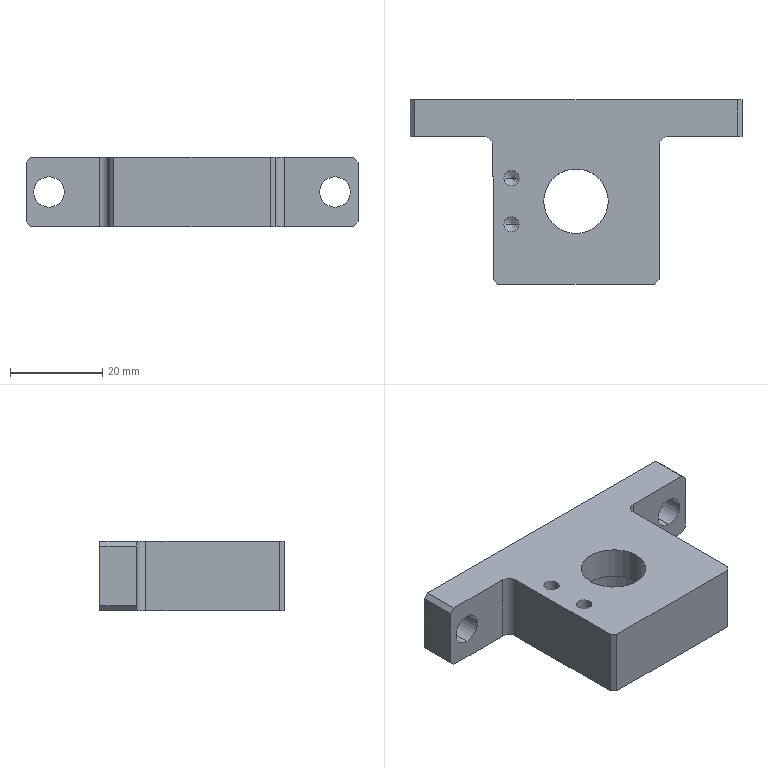Part | STEP file | FBDS-CS-018 | 1 solid | 47 faces | box 72 x 40 x 15 mm | volume 21999 mm3 | cylinder 18 | plane 17 | cone 12 | commonest cylinder face diameters 2.5 x4 3.3 x4 6.6 x4 4 x2 14 x2 18 x2
STEP:
#1=CARTESIAN_POINT('',(12.25,-2.,0.275));
#2=VERTEX_POINT('',#1);
#3=CARTESIAN_POINT('',(9.75,-2.,0.275));
#4=VERTEX_POINT('',#3);
#5=CARTESIAN_POINT('',(11.,-2.,0.275));
#6=DIRECTION('',(0.,0.,-1.));
#7=DIRECTION('',(-1.,0.,0.));
#8=AXIS2_PLACEMENT_3D('',#5,#6,#7);
#9=CIRCLE('',#8,1.25);
#10=EDGE_CURVE('',#2,#4,#9,.T.);
#11=ORIENTED_EDGE('',*,*,#10,.F.);
#12=CARTESIAN_POINT('',(12.525,-2.,0.));
#13=VERTEX_POINT('',#12);
#14=CARTESIAN_POINT('',(12.525,-2.,0.));
#15=DIRECTION('',(0.7071,0.,-0.7071));
#16=VECTOR('',#15,1000.);
#17=LINE('',#14,#16);
#18=EDGE_CURVE('',#2,#13,#17,.T.);
#19=ORIENTED_EDGE('',*,*,#18,.T.);
#20=CARTESIAN_POINT('',(9.475,-2.,0.));
#21=VERTEX_POINT('',#20);
#22=CARTESIAN_POINT('',(11.,-2.,0.));
#23=DIRECTION('',(0.,0.,-1.));
#24=DIRECTION('',(-1.,0.,0.));
#25=AXIS2_PLACEMENT_3D('',#22,#23,#24);
#26=CIRCLE('',#25,1.525);
#27=EDGE_CURVE('',#13,#21,#26,.T.);
#28=ORIENTED_EDGE('',*,*,#27,.T.);
#29=CARTESIAN_POINT('',(9.475,-2.,0.));
#30=DIRECTION('',(-0.7071,0.,-0.7071));
#31=VECTOR('',#30,1000.);
#32=LINE('',#29,#31);
#33=EDGE_CURVE('',#4,#21,#32,.T.);
#34=ORIENTED_EDGE('',*,*,#33,.F.);
#35=EDGE_LOOP('',(#11,#19,#28,#34));
#36=FACE_OUTER_BOUND('',#35,.T.);
#37=CARTESIAN_POINT('',(11.,-2.,0.));
#38=DIRECTION('',(0.,0.,-1.));
#39=DIRECTION('',(-1.,0.,0.));
#40=AXIS2_PLACEMENT_3D('',#37,#38,#39);
#41=CONICAL_SURFACE('',#40,1.525,0.7854);
#42=ADVANCED_FACE('',(#36),#41,.F.);
#43=CARTESIAN_POINT('',(12.25,-2.,7.5));
#44=VERTEX_POINT('',#43);
#45=CARTESIAN_POINT('',(9.75,-2.,7.5));
#46=VERTEX_POINT('',#45);
#47=CARTESIAN_POINT('',(11.,-2.,7.5));
#48=DIRECTION('',(0.,0.,-1.));
#49=DIRECTION('',(-1.,0.,0.));
#50=AXIS2_PLACEMENT_3D('',#47,#48,#49);
#51=CIRCLE('',#50,1.25);
#52=EDGE_CURVE('',#44,#46,#51,.T.);
#53=ORIENTED_EDGE('',*,*,#52,.F.);
#54=CARTESIAN_POINT('',(12.25,-2.,0.));
#55=DIRECTION('',(0.,0.,-1.));
#56=VECTOR('',#55,1000.);
#57=LINE('',#54,#56);
#58=EDGE_CURVE('',#44,#2,#57,.T.);
#59=ORIENTED_EDGE('',*,*,#58,.T.);
#60=ORIENTED_EDGE('',*,*,#10,.T.);
#61=CARTESIAN_POINT('',(9.75,-2.,0.));
#62=DIRECTION('',(0.,0.,-1.));
#63=VECTOR('',#62,1000.);
#64=LINE('',#61,#63);
#65=EDGE_CURVE('',#46,#4,#64,.T.);
#66=ORIENTED_EDGE('',*,*,#65,.F.);
#67=EDGE_LOOP('',(#53,#59,#60,#66));
#68=FACE_OUTER_BOUND('',#67,.T.);
#69=CARTESIAN_POINT('',(11.,-2.,0.));
#70=DIRECTION('',(0.,0.,-1.));
#71=DIRECTION('',(-1.,0.,0.));
#72=AXIS2_PLACEMENT_3D('',#69,#70,#71);
#73=CYLINDRICAL_SURFACE('',#72,1.25);
#74=ADVANCED_FACE('',(#68),#73,.F.);
#75=CARTESIAN_POINT('',(11.,-2.,8.251));
#76=VERTEX_POINT('',#75);
#77=CARTESIAN_POINT('',(9.75,-2.,7.5));
#78=DIRECTION('',(-0.8572,0.,-0.515));
#79=VECTOR('',#78,1000.);
#80=LINE('',#77,#79);
#81=EDGE_CURVE('',#76,#46,#80,.T.);
#82=ORIENTED_EDGE('',*,*,#81,.F.);
#83=CARTESIAN_POINT('',(12.25,-2.,7.5));
#84=DIRECTION('',(0.8572,0.,-0.515));
#85=VECTOR('',#84,1000.);
#86=LINE('',#83,#85);
#87=EDGE_CURVE('',#76,#44,#86,.T.);
#88=ORIENTED_EDGE('',*,*,#87,.T.);
#89=ORIENTED_EDGE('',*,*,#52,.T.);
#90=EDGE_LOOP('',(#82,#88,#89));
#91=FACE_OUTER_BOUND('',#90,.T.);
#92=CARTESIAN_POINT('',(11.,-2.,7.5));
#93=DIRECTION('',(0.,0.,-1.));
#94=DIRECTION('',(-1.,0.,0.));
#95=AXIS2_PLACEMENT_3D('',#92,#93,#94);
#96=CONICAL_SURFACE('',#95,1.25,1.03);
#97=ADVANCED_FACE('',(#91),#96,.F.);
#98=CARTESIAN_POINT('',(-9.75,-2.,0.275));
#99=VERTEX_POINT('',#98);
#100=CARTESIAN_POINT('',(-12.25,-2.,0.275));
#101=VERTEX_POINT('',#100);
#102=CARTESIAN_POINT('',(-11.,-2.,0.275));
#103=DIRECTION('',(0.,0.,-1.));
#104=DIRECTION('',(-1.,0.,0.));
#105=AXIS2_PLACEMENT_3D('',#102,#103,#104);
#106=CIRCLE('',#105,1.25);
#107=EDGE_CURVE('',#99,#101,#106,.T.);
#108=ORIENTED_EDGE('',*,*,#107,.F.);
#109=CARTESIAN_POINT('',(-9.475,-2.,0.));
#110=VERTEX_POINT('',#109);
#111=CARTESIAN_POINT('',(-9.475,-2.,0.));
#112=DIRECTION('',(0.7071,0.,-0.7071));
#113=VECTOR('',#112,1000.);
#114=LINE('',#111,#113);
#115=EDGE_CURVE('',#99,#110,#114,.T.);
#116=ORIENTED_EDGE('',*,*,#115,.T.);
#117=CARTESIAN_POINT('',(-12.525,-2.,0.));
#118=VERTEX_POINT('',#117);
#119=CARTESIAN_POINT('',(-11.,-2.,0.));
#120=DIRECTION('',(0.,0.,-1.));
#121=DIRECTION('',(-1.,0.,0.));
#122=AXIS2_PLACEMENT_3D('',#119,#120,#121);
#123=CIRCLE('',#122,1.525);
#124=EDGE_CURVE('',#110,#118,#123,.T.);
#125=ORIENTED_EDGE('',*,*,#124,.T.);
#126=CARTESIAN_POINT('',(-12.525,-2.,0.));
#127=DIRECTION('',(-0.7071,0.,-0.7071));
#128=VECTOR('',#127,1000.);
#129=LINE('',#126,#128);
#130=EDGE_CURVE('',#101,#118,#129,.T.);
#131=ORIENTED_EDGE('',*,*,#130,.F.);
#132=EDGE_LOOP('',(#108,#116,#125,#131));
#133=FACE_OUTER_BOUND('',#132,.T.);
#134=CARTESIAN_POINT('',(-11.,-2.,0.));
#135=DIRECTION('',(0.,0.,-1.));
#136=DIRECTION('',(-1.,0.,0.));
#137=AXIS2_PLACEMENT_3D('',#134,#135,#136);
#138=CONICAL_SURFACE('',#137,1.525,0.7854);
#139=ADVANCED_FACE('',(#133),#138,.F.);
#140=CARTESIAN_POINT('',(-9.75,-2.,7.5));
#141=VERTEX_POINT('',#140);
#142=CARTESIAN_POINT('',(-12.25,-2.,7.5));
#143=VERTEX_POINT('',#142);
#144=CARTESIAN_POINT('',(-11.,-2.,7.5));
#145=DIRECTION('',(0.,0.,-1.));
#146=DIRECTION('',(-1.,0.,0.));
#147=AXIS2_PLACEMENT_3D('',#144,#145,#146);
#148=CIRCLE('',#147,1.25);
#149=EDGE_CURVE('',#141,#143,#148,.T.);
#150=ORIENTED_EDGE('',*,*,#149,.F.);
#151=CARTESIAN_POINT('',(-9.75,-2.,0.));
#152=DIRECTION('',(0.,0.,-1.));
#153=VECTOR('',#152,1000.);
#154=LINE('',#151,#153);
#155=EDGE_CURVE('',#141,#99,#154,.T.);
#156=ORIENTED_EDGE('',*,*,#155,.T.);
#157=ORIENTED_EDGE('',*,*,#107,.T.);
#158=CARTESIAN_POINT('',(-12.25,-2.,0.));
#159=DIRECTION('',(0.,0.,-1.));
#160=VECTOR('',#159,1000.);
#161=LINE('',#158,#160);
#162=EDGE_CURVE('',#143,#101,#161,.T.);
#163=ORIENTED_EDGE('',*,*,#162,.F.);
#164=EDGE_LOOP('',(#150,#156,#157,#163));
#165=FACE_OUTER_BOUND('',#164,.T.);
#166=CARTESIAN_POINT('',(-11.,-2.,0.));
#167=DIRECTION('',(0.,0.,-1.));
#168=DIRECTION('',(-1.,0.,0.));
#169=AXIS2_PLACEMENT_3D('',#166,#167,#168);
#170=CYLINDRICAL_SURFACE('',#169,1.25);
#171=ADVANCED_FACE('',(#165),#170,.F.);
#172=CARTESIAN_POINT('',(-11.,-2.,8.251));
#173=VERTEX_POINT('',#172);
#174=CARTESIAN_POINT('',(-12.25,-2.,7.5));
#175=DIRECTION('',(-0.8572,0.,-0.515));
#176=VECTOR('',#175,1000.);
#177=LINE('',#174,#176);
#178=EDGE_CURVE('',#173,#143,#177,.T.);
#179=ORIENTED_EDGE('',*,*,#178,.F.);
#180=CARTESIAN_POINT('',(-9.75,-2.,7.5));
#181=DIRECTION('',(0.8572,0.,-0.515));
#182=VECTOR('',#181,1000.);
#183=LINE('',#180,#182);
#184=EDGE_CURVE('',#173,#141,#183,.T.);
#185=ORIENTED_EDGE('',*,*,#184,.T.);
#186=ORIENTED_EDGE('',*,*,#149,.T.);
#187=EDGE_LOOP('',(#179,#185,#186));
#188=FACE_OUTER_BOUND('',#187,.T.);
#189=CARTESIAN_POINT('',(-11.,-2.,7.5));
#190=DIRECTION('',(0.,0.,-1.));
#191=DIRECTION('',(-1.,0.,0.));
#192=AXIS2_PLACEMENT_3D('',#189,#190,#191);
#193=CONICAL_SURFACE('',#192,1.25,1.03);
#194=ADVANCED_FACE('',(#188),#193,.F.);
#195=CARTESIAN_POINT('',(-15.65,3.,4.9));
#196=VERTEX_POINT('',#195);
#197=CARTESIAN_POINT('',(-12.35,3.,4.9));
#198=VERTEX_POINT('',#197);
#199=CARTESIAN_POINT('',(-14.,3.,4.9));
#200=DIRECTION('',(0.,0.,1.));
#201=DIRECTION('',(1.,0.,0.));
#202=AXIS2_PLACEMENT_3D('',#199,#200,#201);
#203=CIRCLE('',#202,1.65);
#204=EDGE_CURVE('',#196,#198,#203,.T.);
#205=ORIENTED_EDGE('',*,*,#204,.F.);
#206=CARTESIAN_POINT('',(-15.65,3.,15.));
#207=VERTEX_POINT('',#206);
#208=CARTESIAN_POINT('',(-15.65,3.,15.));
#209=DIRECTION('',(0.,0.,1.));
#210=VECTOR('',#209,1000.);
#211=LINE('',#208,#210);
#212=EDGE_CURVE('',#196,#207,#211,.T.);
#213=ORIENTED_EDGE('',*,*,#212,.T.);
#214=CARTESIAN_POINT('',(-12.35,3.,15.));
#215=VERTEX_POINT('',#214);
#216=CARTESIAN_POINT('',(-14.,3.,15.));
#217=DIRECTION('',(0.,0.,1.));
#218=DIRECTION('',(1.,0.,0.));
#219=AXIS2_PLACEMENT_3D('',#216,#217,#218);
#220=CIRCLE('',#219,1.65);
#221=EDGE_CURVE('',#207,#215,#220,.T.);
#222=ORIENTED_EDGE('',*,*,#221,.T.);
#223=CARTESIAN_POINT('',(-12.35,3.,15.));
#224=DIRECTION('',(0.,0.,1.));
#225=VECTOR('',#224,1000.);
#226=LINE('',#223,#225);
#227=EDGE_CURVE('',#198,#215,#226,.T.);
#228=ORIENTED_EDGE('',*,*,#227,.F.);
#229=EDGE_LOOP('',(#205,#213,#222,#228));
#230=FACE_OUTER_BOUND('',#229,.T.);
#231=CARTESIAN_POINT('',(-14.,3.,15.));
#232=DIRECTION('',(0.,0.,1.));
#233=DIRECTION('',(1.,0.,0.));
#234=AXIS2_PLACEMENT_3D('',#231,#232,#233);
#235=CYLINDRICAL_SURFACE('',#234,1.65);
#236=ADVANCED_FACE('',(#230),#235,.F.);
#237=CARTESIAN_POINT('',(-14.,3.,3.909));
#238=VERTEX_POINT('',#237);
#239=CARTESIAN_POINT('',(-12.35,3.,4.9));
#240=DIRECTION('',(0.8572,0.,0.515));
#241=VECTOR('',#240,1000.);
#242=LINE('',#239,#241);
#243=EDGE_CURVE('',#238,#198,#242,.T.);
#244=ORIENTED_EDGE('',*,*,#243,.F.);
#245=CARTESIAN_POINT('',(-15.65,3.,4.9));
#246=DIRECTION('',(-0.8572,0.,0.515));
#247=VECTOR('',#246,1000.);
#248=LINE('',#245,#247);
#249=EDGE_CURVE('',#238,#196,#248,.T.);
#250=ORIENTED_EDGE('',*,*,#249,.T.);
#251=ORIENTED_EDGE('',*,*,#204,.T.);
#252=EDGE_LOOP('',(#244,#250,#251));
#253=FACE_OUTER_BOUND('',#252,.T.);
#254=CARTESIAN_POINT('',(-14.,3.,4.9));
#255=DIRECTION('',(0.,0.,1.));
#256=DIRECTION('',(1.,0.,0.));
#257=AXIS2_PLACEMENT_3D('',#254,#255,#256);
#258=CONICAL_SURFACE('',#257,1.65,1.03);
#259=ADVANCED_FACE('',(#253),#258,.F.);
#260=CARTESIAN_POINT('',(-15.65,-7.,4.9));
#261=VERTEX_POINT('',#260);
#262=CARTESIAN_POINT('',(-12.35,-7.,4.9));
#263=VERTEX_POINT('',#262);
#264=CARTESIAN_POINT('',(-14.,-7.,4.9));
#265=DIRECTION('',(0.,0.,1.));
#266=DIRECTION('',(1.,0.,0.));
#267=AXIS2_PLACEMENT_3D('',#264,#265,#266);
#268=CIRCLE('',#267,1.65);
#269=EDGE_CURVE('',#261,#263,#268,.T.);
#270=ORIENTED_EDGE('',*,*,#269,.F.);
#271=CARTESIAN_POINT('',(-15.65,-7.,15.));
#272=VERTEX_POINT('',#271);
#273=CARTESIAN_POINT('',(-15.65,-7.,15.));
#274=DIRECTION('',(0.,0.,1.));
#275=VECTOR('',#274,1000.);
#276=LINE('',#273,#275);
#277=EDGE_CURVE('',#261,#272,#276,.T.);
#278=ORIENTED_EDGE('',*,*,#277,.T.);
#279=CARTESIAN_POINT('',(-12.35,-7.,15.));
#280=VERTEX_POINT('',#279);
#281=CARTESIAN_POINT('',(-14.,-7.,15.));
#282=DIRECTION('',(0.,0.,1.));
#283=DIRECTION('',(1.,0.,0.));
#284=AXIS2_PLACEMENT_3D('',#281,#282,#283);
#285=CIRCLE('',#284,1.65);
#286=EDGE_CURVE('',#272,#280,#285,.T.);
#287=ORIENTED_EDGE('',*,*,#286,.T.);
#288=CARTESIAN_POINT('',(-12.35,-7.,15.));
#289=DIRECTION('',(0.,0.,1.));
#290=VECTOR('',#289,1000.);
#291=LINE('',#288,#290);
#292=EDGE_CURVE('',#263,#280,#291,.T.);
#293=ORIENTED_EDGE('',*,*,#292,.F.);
#294=EDGE_LOOP('',(#270,#278,#287,#293));
#295=FACE_OUTER_BOUND('',#294,.T.);
#296=CARTESIAN_POINT('',(-14.,-7.,15.));
#297=DIRECTION('',(0.,0.,1.));
#298=DIRECTION('',(1.,0.,0.));
#299=AXIS2_PLACEMENT_3D('',#296,#297,#298);
#300=CYLINDRICAL_SURFACE('',#299,1.65);
#301=ADVANCED_FACE('',(#295),#300,.F.);
#302=CARTESIAN_POINT('',(-14.,-7.,3.909));
#303=VERTEX_POINT('',#302);
#304=CARTESIAN_POINT('',(-12.35,-7.,4.9));
#305=DIRECTION('',(0.8572,0.,0.515));
#306=VECTOR('',#305,1000.);
#307=LINE('',#304,#306);
#308=EDGE_CURVE('',#303,#263,#307,.T.);
#309=ORIENTED_EDGE('',*,*,#308,.F.);
#310=CARTESIAN_POINT('',(-15.65,-7.,4.9));
#311=DIRECTION('',(-0.8572,0.,0.515));
#312=VECTOR('',#311,1000.);
#313=LINE('',#310,#312);
#314=EDGE_CURVE('',#303,#261,#313,.T.);
#315=ORIENTED_EDGE('',*,*,#314,.T.);
#316=ORIENTED_EDGE('',*,*,#269,.T.);
#317=EDGE_LOOP('',(#309,#315,#316));
#318=FACE_OUTER_BOUND('',#317,.T.);
#319=CARTESIAN_POINT('',(-14.,-7.,4.9));
#320=DIRECTION('',(0.,0.,1.));
#321=DIRECTION('',(1.,0.,0.));
#322=AXIS2_PLACEMENT_3D('',#319,#320,#321);
#323=CONICAL_SURFACE('',#322,1.65,1.03);
#324=ADVANCED_FACE('',(#318),#323,.F.);
#325=CARTESIAN_POINT('',(-31.,20.,10.8));
#326=VERTEX_POINT('',#325);
#327=CARTESIAN_POINT('',(-31.,20.,4.2));
#328=VERTEX_POINT('',#327);
#329=CARTESIAN_POINT('',(-31.,20.,7.5));
#330=DIRECTION('',(0.,-1.,0.));
#331=DIRECTION('',(0.,0.,-1.));
#332=AXIS2_PLACEMENT_3D('',#329,#330,#331);
#333=CIRCLE('',#332,3.3);
#334=EDGE_CURVE('',#326,#328,#333,.T.);
#335=ORIENTED_EDGE('',*,*,#334,.F.);
#336=CARTESIAN_POINT('',(-31.,12.,10.8));
#337=VERTEX_POINT('',#336);
#338=CARTESIAN_POINT('',(-31.,12.,10.8));
#339=DIRECTION('',(0.,-1.,0.));
#340=VECTOR('',#339,1000.);
#341=LINE('',#338,#340);
#342=EDGE_CURVE('',#326,#337,#341,.T.);
#343=ORIENTED_EDGE('',*,*,#342,.T.);
#344=CARTESIAN_POINT('',(-31.,12.,4.2));
#345=VERTEX_POINT('',#344);
#346=CARTESIAN_POINT('',(-31.,12.,7.5));
#347=DIRECTION('',(0.,-1.,0.));
#348=DIRECTION('',(0.,0.,-1.));
#349=AXIS2_PLACEMENT_3D('',#346,#347,#348);
#350=CIRCLE('',#349,3.3);
#351=EDGE_CURVE('',#337,#345,#350,.T.);
#352=ORIENTED_EDGE('',*,*,#351,.T.);
#353=CARTESIAN_POINT('',(-31.,12.,4.2));
#354=DIRECTION('',(0.,-1.,0.));
#355=VECTOR('',#354,1000.);
#356=LINE('',#353,#355);
#357=EDGE_CURVE('',#328,#345,#356,.T.);
#358=ORIENTED_EDGE('',*,*,#357,.F.);
#359=EDGE_LOOP('',(#335,#343,#352,#358));
#360=FACE_OUTER_BOUND('',#359,.T.);
#361=CARTESIAN_POINT('',(-31.,12.,7.5));
#362=DIRECTION('',(0.,-1.,0.));
#363=DIRECTION('',(0.,0.,-1.));
#364=AXIS2_PLACEMENT_3D('',#361,#362,#363);
#365=CYLINDRICAL_SURFACE('',#364,3.3);
#366=ADVANCED_FACE('',(#360),#365,.F.);
#367=CARTESIAN_POINT('',(31.,20.,10.8));
#368=VERTEX_POINT('',#367);
#369=CARTESIAN_POINT('',(31.,20.,4.2));
#370=VERTEX_POINT('',#369);
#371=CARTESIAN_POINT('',(31.,20.,7.5));
#372=DIRECTION('',(0.,-1.,0.));
#373=DIRECTION('',(0.,0.,-1.));
#374=AXIS2_PLACEMENT_3D('',#371,#372,#373);
#375=CIRCLE('',#374,3.3);
#376=EDGE_CURVE('',#368,#370,#375,.T.);
#377=ORIENTED_EDGE('',*,*,#376,.F.);
#378=CARTESIAN_POINT('',(31.,12.,10.8));
#379=VERTEX_POINT('',#378);
#380=CARTESIAN_POINT('',(31.,12.,10.8));
#381=DIRECTION('',(0.,-1.,0.));
#382=VECTOR('',#381,1000.);
#383=LINE('',#380,#382);
#384=EDGE_CURVE('',#368,#379,#383,.T.);
#385=ORIENTED_EDGE('',*,*,#384,.T.);
#386=CARTESIAN_POINT('',(31.,12.,4.2));
#387=VERTEX_POINT('',#386);
#388=CARTESIAN_POINT('',(31.,12.,7.5));
#389=DIRECTION('',(0.,-1.,0.));
#390=DIRECTION('',(0.,0.,-1.));
#391=AXIS2_PLACEMENT_3D('',#388,#389,#390);
#392=CIRCLE('',#391,3.3);
#393=EDGE_CURVE('',#379,#387,#392,.T.);
#394=ORIENTED_EDGE('',*,*,#393,.T.);
#395=CARTESIAN_POINT('',(31.,12.,4.2));
#396=DIRECTION('',(0.,-1.,0.));
#397=VECTOR('',#396,1000.);
#398=LINE('',#395,#397);
#399=EDGE_CURVE('',#370,#387,#398,.T.);
#400=ORIENTED_EDGE('',*,*,#399,.F.);
#401=EDGE_LOOP('',(#377,#385,#394,#400));
#402=FACE_OUTER_BOUND('',#401,.T.);
#403=CARTESIAN_POINT('',(31.,12.,7.5));
#404=DIRECTION('',(0.,-1.,0.));
#405=DIRECTION('',(0.,0.,-1.));
#406=AXIS2_PLACEMENT_3D('',#403,#404,#405);
#407=CYLINDRICAL_SURFACE('',#406,3.3);
#408=ADVANCED_FACE('',(#402),#407,.F.);
#409=CARTESIAN_POINT('',(7.,-2.,15.));
#410=VERTEX_POINT('',#409);
#411=CARTESIAN_POINT('',(-7.,-2.,15.));
#412=VERTEX_POINT('',#411);
#413=CARTESIAN_POINT('',(0.,-2.,15.));
#414=DIRECTION('',(0.,0.,-1.));
#415=DIRECTION('',(-1.,0.,0.));
#416=AXIS2_PLACEMENT_3D('',#413,#414,#415);
#417=CIRCLE('',#416,7.);
#418=EDGE_CURVE('',#410,#412,#417,.T.);
#419=ORIENTED_EDGE('',*,*,#418,.F.);
#420=CARTESIAN_POINT('',(7.,-2.,8.));
#421=VERTEX_POINT('',#420);
#422=CARTESIAN_POINT('',(7.,-2.,18.));
#423=DIRECTION('',(0.,0.,-1.));
#424=VECTOR('',#423,1000.);
#425=LINE('',#422,#424);
#426=EDGE_CURVE('',#410,#421,#425,.T.);
#427=ORIENTED_EDGE('',*,*,#426,.T.);
#428=CARTESIAN_POINT('',(-7.,-2.,8.));
#429=VERTEX_POINT('',#428);
#430=CARTESIAN_POINT('',(0.,-2.,8.));
#431=DIRECTION('',(0.,0.,-1.));
#432=DIRECTION('',(-1.,0.,0.));
#433=AXIS2_PLACEMENT_3D('',#430,#431,#432);
#434=CIRCLE('',#433,7.);
#435=EDGE_CURVE('',#421,#429,#434,.T.);
#436=ORIENTED_EDGE('',*,*,#435,.T.);
#437=CARTESIAN_POINT('',(-7.,-2.,18.));
#438=DIRECTION('',(0.,0.,-1.));
#439=VECTOR('',#438,1000.);
#440=LINE('',#437,#439);
#441=EDGE_CURVE('',#412,#429,#440,.T.);
#442=ORIENTED_EDGE('',*,*,#441,.F.);
#443=EDGE_LOOP('',(#419,#427,#436,#442));
#444=FACE_OUTER_BOUND('',#443,.T.);
#445=CARTESIAN_POINT('',(0.,-2.,18.));
#446=DIRECTION('',(0.,0.,-1.));
#447=DIRECTION('',(-1.,0.,0.));
#448=AXIS2_PLACEMENT_3D('',#445,#446,#447);
#449=CYLINDRICAL_SURFACE('',#448,7.);
#450=ADVANCED_FACE('',(#444),#449,.F.);
#451=CARTESIAN_POINT('',(-9.,-2.,8.));
#452=VERTEX_POINT('',#451);
#453=CARTESIAN_POINT('',(9.,-2.,8.));
#454=VERTEX_POINT('',#453);
#455=CARTESIAN_POINT('',(0.,-2.,8.));
#456=DIRECTION('',(0.,0.,1.));
#457=DIRECTION('',(1.,0.,0.));
#458=AXIS2_PLACEMENT_3D('',#455,#456,#457);
#459=CIRCLE('',#458,9.);
#460=EDGE_CURVE('',#452,#454,#459,.T.);
#461=ORIENTED_EDGE('',*,*,#460,.T.);
#462=CARTESIAN_POINT('',(9.,-2.,0.));
#463=VERTEX_POINT('',#462);
#464=CARTESIAN_POINT('',(9.,-2.,8.));
#465=DIRECTION('',(0.,0.,-1.));
#466=VECTOR('',#465,1000.);
#467=LINE('',#464,#466);
#468=EDGE_CURVE('',#454,#463,#467,.T.);
#469=ORIENTED_EDGE('',*,*,#468,.T.);
#470=CARTESIAN_POINT('',(-9.,-2.,0.));
#471=VERTEX_POINT('',#470);
#472=CARTESIAN_POINT('',(0.,-2.,0.));
#473=DIRECTION('',(0.,0.,1.));
#474=DIRECTION('',(1.,0.,0.));
#475=AXIS2_PLACEMENT_3D('',#472,#473,#474);
#476=CIRCLE('',#475,9.);
#477=EDGE_CURVE('',#471,#463,#476,.T.);
#478=ORIENTED_EDGE('',*,*,#477,.F.);
#479=CARTESIAN_POINT('',(-9.,-2.,8.));
#480=DIRECTION('',(0.,0.,-1.));
#481=VECTOR('',#480,1000.);
#482=LINE('',#479,#481);
#483=EDGE_CURVE('',#452,#471,#482,.T.);
#484=ORIENTED_EDGE('',*,*,#483,.F.);
#485=EDGE_LOOP('',(#461,#469,#478,#484));
#486=FACE_OUTER_BOUND('',#485,.T.);
#487=CARTESIAN_POINT('',(0.,-2.,8.));
#488=DIRECTION('',(0.,0.,-1.));
#489=DIRECTION('',(-1.,0.,0.));
#490=AXIS2_PLACEMENT_3D('',#487,#488,#489);
#491=CYLINDRICAL_SURFACE('',#490,9.);
#492=ADVANCED_FACE('',(#486),#491,.F.);
#493=CARTESIAN_POINT('',(36.,12.,1.));
#494=VERTEX_POINT('',#493);
#495=CARTESIAN_POINT('',(36.,12.,14.));
#496=VERTEX_POINT('',#495);
#497=CARTESIAN_POINT('',(36.,12.,-3.));
#498=DIRECTION('',(0.,0.,1.));
#499=VECTOR('',#498,1000.);
#500=LINE('',#497,#499);
#501=EDGE_CURVE('',#494,#496,#500,.T.);
#502=ORIENTED_EDGE('',*,*,#501,.F.);
#503=CARTESIAN_POINT('',(36.,20.,1.));
#504=VERTEX_POINT('',#503);
#505=CARTESIAN_POINT('',(36.,20.,1.));
#506=DIRECTION('',(0.,1.,0.));
#507=VECTOR('',#506,1000.);
#508=LINE('',#505,#507);
#509=EDGE_CURVE('',#494,#504,#508,.T.);
#510=ORIENTED_EDGE('',*,*,#509,.T.);
#511=CARTESIAN_POINT('',(36.,20.,14.));
#512=VERTEX_POINT('',#511);
#513=CARTESIAN_POINT('',(36.,20.,15.));
#514=DIRECTION('',(0.,0.,-1.));
#515=VECTOR('',#514,1000.);
#516=LINE('',#513,#515);
#517=EDGE_CURVE('',#512,#504,#516,.T.);
#518=ORIENTED_EDGE('',*,*,#517,.F.);
#519=CARTESIAN_POINT('',(36.,-20.,14.));
#520=DIRECTION('',(0.,-1.,0.));
#521=VECTOR('',#520,1000.);
#522=LINE('',#519,#521);
#523=EDGE_CURVE('',#512,#496,#522,.T.);
#524=ORIENTED_EDGE('',*,*,#523,.T.);
#525=EDGE_LOOP('',(#502,#510,#518,#524));
#526=FACE_OUTER_BOUND('',#525,.T.);
#527=CARTESIAN_POINT('',(36.,-20.,15.));
#528=DIRECTION('',(-1.,0.,0.));
#529=DIRECTION('',(0.,0.,1.));
#530=AXIS2_PLACEMENT_3D('',#527,#528,#529);
#531=PLANE('',#530);
#532=ADVANCED_FACE('',(#526),#531,.F.);
#533=CARTESIAN_POINT('',(-31.,20.,7.5));
#534=DIRECTION('',(0.,-1.,0.));
#535=DIRECTION('',(0.,0.,-1.));
#536=AXIS2_PLACEMENT_3D('',#533,#534,#535);
#537=CIRCLE('',#536,3.3);
#538=EDGE_CURVE('',#328,#326,#537,.T.);
#539=ORIENTED_EDGE('',*,*,#538,.T.);
#540=ORIENTED_EDGE('',*,*,#334,.T.);
#541=EDGE_LOOP('',(#539,#540));
#542=FACE_BOUND('',#541,.T.);
#543=CARTESIAN_POINT('',(31.,20.,7.5));
#544=DIRECTION('',(0.,-1.,0.));
#545=DIRECTION('',(0.,0.,-1.));
#546=AXIS2_PLACEMENT_3D('',#543,#544,#545);
#547=CIRCLE('',#546,3.3);
#548=EDGE_CURVE('',#370,#368,#547,.T.);
#549=ORIENTED_EDGE('',*,*,#548,.T.);
#550=ORIENTED_EDGE('',*,*,#376,.T.);
#551=EDGE_LOOP('',(#549,#550));
#552=FACE_BOUND('',#551,.T.);
#553=ORIENTED_EDGE('',*,*,#517,.T.);
#554=CARTESIAN_POINT('',(35.,20.,0.));
#555=VERTEX_POINT('',#554);
#556=CARTESIAN_POINT('',(36.,20.,1.));
#557=DIRECTION('',(-0.7071,0.,-0.7071));
#558=VECTOR('',#557,1000.);
#559=LINE('',#556,#558);
#560=EDGE_CURVE('',#504,#555,#559,.T.);
#561=ORIENTED_EDGE('',*,*,#560,.T.);
#562=CARTESIAN_POINT('',(-35.,20.,0.));
#563=VERTEX_POINT('',#562);
#564=CARTESIAN_POINT('',(-36.,20.,0.));
#565=DIRECTION('',(-1.,0.,0.));
#566=VECTOR('',#565,1000.);
#567=LINE('',#564,#566);
#568=EDGE_CURVE('',#555,#563,#567,.T.);
#569=ORIENTED_EDGE('',*,*,#568,.T.);
#570=CARTESIAN_POINT('',(-36.,20.,1.));
#571=VERTEX_POINT('',#570);
#572=CARTESIAN_POINT('',(-36.,20.,1.));
#573=DIRECTION('',(-0.7071,0.,0.7071));
#574=VECTOR('',#573,1000.);
#575=LINE('',#572,#574);
#576=EDGE_CURVE('',#563,#571,#575,.T.);
#577=ORIENTED_EDGE('',*,*,#576,.T.);
#578=CARTESIAN_POINT('',(-36.,20.,14.));
#579=VERTEX_POINT('',#578);
#580=CARTESIAN_POINT('',(-36.,20.,15.));
#581=DIRECTION('',(0.,0.,-1.));
#582=VECTOR('',#581,1000.);
#583=LINE('',#580,#582);
#584=EDGE_CURVE('',#579,#571,#583,.T.);
#585=ORIENTED_EDGE('',*,*,#584,.F.);
#586=CARTESIAN_POINT('',(-35.,20.,15.));
#587=VERTEX_POINT('',#586);
#588=CARTESIAN_POINT('',(-35.,20.,15.));
#589=DIRECTION('',(0.7071,0.,0.7071));
#590=VECTOR('',#589,1000.);
#591=LINE('',#588,#590);
#592=EDGE_CURVE('',#579,#587,#591,.T.);
#593=ORIENTED_EDGE('',*,*,#592,.T.);
#594=CARTESIAN_POINT('',(35.,20.,15.));
#595=VERTEX_POINT('',#594);
#596=CARTESIAN_POINT('',(-36.,20.,15.));
#597=DIRECTION('',(-1.,0.,0.));
#598=VECTOR('',#597,1000.);
#599=LINE('',#596,#598);
#600=EDGE_CURVE('',#595,#587,#599,.T.);
#601=ORIENTED_EDGE('',*,*,#600,.F.);
#602=CARTESIAN_POINT('',(35.,20.,15.));
#603=DIRECTION('',(0.7071,0.,-0.7071));
#604=VECTOR('',#603,1000.);
#605=LINE('',#602,#604);
#606=EDGE_CURVE('',#595,#512,#605,.T.);
#607=ORIENTED_EDGE('',*,*,#606,.T.);
#608=EDGE_LOOP('',(#553,#561,#569,#577,#585,#593,#601,#607));
#609=FACE_OUTER_BOUND('',#608,.T.);
#610=CARTESIAN_POINT('',(-36.,20.,15.));
#611=DIRECTION('',(0.,-1.,0.));
#612=DIRECTION('',(0.,0.,-1.));
#613=AXIS2_PLACEMENT_3D('',#610,#611,#612);
#614=PLANE('',#613);
#615=ADVANCED_FACE('',(#542,#552,#609),#614,.F.);
#616=ORIENTED_EDGE('',*,*,#584,.T.);
#617=CARTESIAN_POINT('',(-36.,12.,1.));
#618=VERTEX_POINT('',#617);
#619=CARTESIAN_POINT('',(-36.,12.,1.));
#620=DIRECTION('',(0.,-1.,0.));
#621=VECTOR('',#620,1000.);
#622=LINE('',#619,#621);
#623=EDGE_CURVE('',#571,#618,#622,.T.);
#624=ORIENTED_EDGE('',*,*,#623,.T.);
#625=CARTESIAN_POINT('',(-36.,12.,14.));
#626=VERTEX_POINT('',#625);
#627=CARTESIAN_POINT('',(-36.,12.,-3.));
#628=DIRECTION('',(0.,0.,1.));
#629=VECTOR('',#628,1000.);
#630=LINE('',#627,#629);
#631=EDGE_CURVE('',#618,#626,#630,.T.);
#632=ORIENTED_EDGE('',*,*,#631,.T.);
#633=CARTESIAN_POINT('',(-36.,-20.,14.));
#634=DIRECTION('',(0.,1.,0.));
#635=VECTOR('',#634,1000.);
#636=LINE('',#633,#635);
#637=EDGE_CURVE('',#626,#579,#636,.T.);
#638=ORIENTED_EDGE('',*,*,#637,.T.);
#639=EDGE_LOOP('',(#616,#624,#632,#638));
#640=FACE_OUTER_BOUND('',#639,.T.);
#641=CARTESIAN_POINT('',(-36.,-20.,15.));
#642=DIRECTION('',(1.,0.,0.));
#643=DIRECTION('',(0.,0.,-1.));
#644=AXIS2_PLACEMENT_3D('',#641,#642,#643);
#645=PLANE('',#644);
#646=ADVANCED_FACE('',(#640),#645,.F.);
#647=CARTESIAN_POINT('',(-17.,-20.,15.));
#648=VERTEX_POINT('',#647);
#649=CARTESIAN_POINT('',(17.,-20.,15.));
#650=VERTEX_POINT('',#649);
#651=CARTESIAN_POINT('',(-36.,-20.,15.));
#652=DIRECTION('',(1.,0.,0.));
#653=VECTOR('',#652,1000.);
#654=LINE('',#651,#653);
#655=EDGE_CURVE('',#648,#650,#654,.T.);
#656=ORIENTED_EDGE('',*,*,#655,.F.);
#657=CARTESIAN_POINT('',(-17.,-20.,0.));
#658=VERTEX_POINT('',#657);
#659=CARTESIAN_POINT('',(-17.,-20.,15.));
#660=DIRECTION('',(0.,0.,-1.));
#661=VECTOR('',#660,1000.);
#662=LINE('',#659,#661);
#663=EDGE_CURVE('',#648,#658,#662,.T.);
#664=ORIENTED_EDGE('',*,*,#663,.T.);
#665=CARTESIAN_POINT('',(17.,-20.,0.));
#666=VERTEX_POINT('',#665);
#667=CARTESIAN_POINT('',(-36.,-20.,0.));
#668=DIRECTION('',(1.,0.,0.));
#669=VECTOR('',#668,1000.);
#670=LINE('',#667,#669);
#671=EDGE_CURVE('',#658,#666,#670,.T.);
#672=ORIENTED_EDGE('',*,*,#671,.T.);
#673=CARTESIAN_POINT('',(17.,-20.,15.));
#674=DIRECTION('',(0.,0.,1.));
#675=VECTOR('',#674,1000.);
#676=LINE('',#673,#675);
#677=EDGE_CURVE('',#666,#650,#676,.T.);
#678=ORIENTED_EDGE('',*,*,#677,.T.);
#679=EDGE_LOOP('',(#656,#664,#672,#678));
#680=FACE_OUTER_BOUND('',#679,.T.);
#681=CARTESIAN_POINT('',(-36.,-20.,15.));
#682=DIRECTION('',(0.,1.,0.));
#683=DIRECTION('',(0.,0.,1.));
#684=AXIS2_PLACEMENT_3D('',#681,#682,#683);
#685=PLANE('',#684);
#686=ADVANCED_FACE('',(#680),#685,.F.);
#687=CARTESIAN_POINT('',(-14.,3.,15.));
#688=DIRECTION('',(0.,0.,1.));
#689=DIRECTION('',(1.,0.,0.));
#690=AXIS2_PLACEMENT_3D('',#687,#688,#689);
#691=CIRCLE('',#690,1.65);
#692=EDGE_CURVE('',#215,#207,#691,.T.);
#693=ORIENTED_EDGE('',*,*,#692,.F.);
#694=ORIENTED_EDGE('',*,*,#221,.F.);
#695=EDGE_LOOP('',(#693,#694));
#696=FACE_BOUND('',#695,.T.);
#697=CARTESIAN_POINT('',(-14.,-7.,15.));
#698=DIRECTION('',(0.,0.,1.));
#699=DIRECTION('',(1.,0.,0.));
#700=AXIS2_PLACEMENT_3D('',#697,#698,#699);
#701=CIRCLE('',#700,1.65);
#702=EDGE_CURVE('',#280,#272,#701,.T.);
#703=ORIENTED_EDGE('',*,*,#702,.F.);
#704=ORIENTED_EDGE('',*,*,#286,.F.);
#705=EDGE_LOOP('',(#703,#704));
#706=FACE_BOUND('',#705,.T.);
#707=CARTESIAN_POINT('',(0.,-2.,15.));
#708=DIRECTION('',(0.,0.,-1.));
#709=DIRECTION('',(-1.,0.,0.));
#710=AXIS2_PLACEMENT_3D('',#707,#708,#709);
#711=CIRCLE('',#710,7.);
#712=EDGE_CURVE('',#412,#410,#711,.T.);
#713=ORIENTED_EDGE('',*,*,#712,.T.);
#714=ORIENTED_EDGE('',*,*,#418,.T.);
#715=EDGE_LOOP('',(#713,#714));
#716=FACE_BOUND('',#715,.T.);
#717=CARTESIAN_POINT('',(-18.,-19.,15.));
#718=VERTEX_POINT('',#717);
#719=CARTESIAN_POINT('',(-18.,10.,15.));
#720=VERTEX_POINT('',#719);
#721=CARTESIAN_POINT('',(-18.,-20.,15.));
#722=DIRECTION('',(0.,1.,0.));
#723=VECTOR('',#722,1000.);
#724=LINE('',#721,#723);
#725=EDGE_CURVE('',#718,#720,#724,.T.);
#726=ORIENTED_EDGE('',*,*,#725,.F.);
#727=CARTESIAN_POINT('',(-18.,-19.,15.));
#728=DIRECTION('',(0.7071,-0.7071,0.));
#729=VECTOR('',#728,1000.);
#730=LINE('',#727,#729);
#731=EDGE_CURVE('',#718,#648,#730,.T.);
#732=ORIENTED_EDGE('',*,*,#731,.T.);
#733=ORIENTED_EDGE('',*,*,#655,.T.);
#734=CARTESIAN_POINT('',(18.,-19.,15.));
#735=VERTEX_POINT('',#734);
#736=CARTESIAN_POINT('',(17.,-20.,15.));
#737=DIRECTION('',(0.7071,0.7071,0.));
#738=VECTOR('',#737,1000.);
#739=LINE('',#736,#738);
#740=EDGE_CURVE('',#650,#735,#739,.T.);
#741=ORIENTED_EDGE('',*,*,#740,.T.);
#742=CARTESIAN_POINT('',(18.,10.,15.));
#743=VERTEX_POINT('',#742);
#744=CARTESIAN_POINT('',(18.,-20.,15.));
#745=DIRECTION('',(0.,-1.,0.));
#746=VECTOR('',#745,1000.);
#747=LINE('',#744,#746);
#748=EDGE_CURVE('',#743,#735,#747,.T.);
#749=ORIENTED_EDGE('',*,*,#748,.F.);
#750=CARTESIAN_POINT('',(20.,12.,15.));
#751=VERTEX_POINT('',#750);
#752=CARTESIAN_POINT('',(20.,10.,15.));
#753=DIRECTION('',(0.,0.,-1.));
#754=DIRECTION('',(-1.,0.,0.));
#755=AXIS2_PLACEMENT_3D('',#752,#753,#754);
#756=CIRCLE('',#755,2.);
#757=EDGE_CURVE('',#743,#751,#756,.T.);
#758=ORIENTED_EDGE('',*,*,#757,.T.);
#759=CARTESIAN_POINT('',(35.,12.,15.));
#760=VERTEX_POINT('',#759);
#761=CARTESIAN_POINT('',(36.,12.,15.));
#762=DIRECTION('',(-1.,0.,0.));
#763=VECTOR('',#762,1000.);
#764=LINE('',#761,#763);
#765=EDGE_CURVE('',#760,#751,#764,.T.);
#766=ORIENTED_EDGE('',*,*,#765,.F.);
#767=CARTESIAN_POINT('',(35.,0.,15.));
#768=DIRECTION('',(0.,1.,0.));
#769=VECTOR('',#768,1000.);
#770=LINE('',#767,#769);
#771=EDGE_CURVE('',#760,#595,#770,.T.);
#772=ORIENTED_EDGE('',*,*,#771,.T.);
#773=ORIENTED_EDGE('',*,*,#600,.T.);
#774=CARTESIAN_POINT('',(-35.,12.,15.));
#775=VERTEX_POINT('',#774);
#776=CARTESIAN_POINT('',(-35.,0.,15.));
#777=DIRECTION('',(0.,-1.,0.));
#778=VECTOR('',#777,1000.);
#779=LINE('',#776,#778);
#780=EDGE_CURVE('',#587,#775,#779,.T.);
#781=ORIENTED_EDGE('',*,*,#780,.T.);
#782=CARTESIAN_POINT('',(-20.,12.,15.));
#783=VERTEX_POINT('',#782);
#784=CARTESIAN_POINT('',(-36.,12.,15.));
#785=DIRECTION('',(-1.,0.,0.));
#786=VECTOR('',#785,1000.);
#787=LINE('',#784,#786);
#788=EDGE_CURVE('',#783,#775,#787,.T.);
#789=ORIENTED_EDGE('',*,*,#788,.F.);
#790=CARTESIAN_POINT('',(-20.,10.,15.));
#791=DIRECTION('',(0.,0.,-1.));
#792=DIRECTION('',(-1.,0.,0.));
#793=AXIS2_PLACEMENT_3D('',#790,#791,#792);
#794=CIRCLE('',#793,2.);
#795=EDGE_CURVE('',#783,#720,#794,.T.);
#796=ORIENTED_EDGE('',*,*,#795,.T.);
#797=EDGE_LOOP('',(#726,#732,#733,#741,#749,#758,#766,#772,#773,#781,#789,#796));
#798=FACE_OUTER_BOUND('',#797,.T.);
#799=CARTESIAN_POINT('',(0.,0.,15.));
#800=DIRECTION('',(0.,0.,-1.));
#801=DIRECTION('',(-1.,0.,0.));
#802=AXIS2_PLACEMENT_3D('',#799,#800,#801);
#803=PLANE('',#802);
#804=ADVANCED_FACE('',(#696,#706,#716,#798),#803,.F.);
#805=CARTESIAN_POINT('',(11.,-2.,0.));
#806=DIRECTION('',(0.,0.,-1.));
#807=DIRECTION('',(-1.,0.,0.));
#808=AXIS2_PLACEMENT_3D('',#805,#806,#807);
#809=CIRCLE('',#808,1.525);
#810=EDGE_CURVE('',#21,#13,#809,.T.);
#811=ORIENTED_EDGE('',*,*,#810,.F.);
#812=ORIENTED_EDGE('',*,*,#27,.F.);
#813=EDGE_LOOP('',(#811,#812));
#814=FACE_BOUND('',#813,.T.);
#815=CARTESIAN_POINT('',(-11.,-2.,0.));
#816=DIRECTION('',(0.,0.,-1.));
#817=DIRECTION('',(-1.,0.,0.));
#818=AXIS2_PLACEMENT_3D('',#815,#816,#817);
#819=CIRCLE('',#818,1.525);
#820=EDGE_CURVE('',#118,#110,#819,.T.);
#821=ORIENTED_EDGE('',*,*,#820,.F.);
#822=ORIENTED_EDGE('',*,*,#124,.F.);
#823=EDGE_LOOP('',(#821,#822));
#824=FACE_BOUND('',#823,.T.);
#825=ORIENTED_EDGE('',*,*,#477,.T.);
#826=CARTESIAN_POINT('',(0.,-2.,0.));
#827=DIRECTION('',(0.,0.,1.));
#828=DIRECTION('',(1.,0.,0.));
#829=AXIS2_PLACEMENT_3D('',#826,#827,#828);
#830=CIRCLE('',#829,9.);
#831=EDGE_CURVE('',#463,#471,#830,.T.);
#832=ORIENTED_EDGE('',*,*,#831,.T.);
#833=EDGE_LOOP('',(#825,#832));
#834=FACE_BOUND('',#833,.T.);
#835=ORIENTED_EDGE('',*,*,#671,.F.);
#836=CARTESIAN_POINT('',(-18.,-19.,0.));
#837=VERTEX_POINT('',#836);
#838=CARTESIAN_POINT('',(-18.5,-18.5,0.));
#839=DIRECTION('',(-0.7071,0.7071,0.));
#840=VECTOR('',#839,1000.);
#841=LINE('',#838,#840);
#842=EDGE_CURVE('',#658,#837,#841,.T.);
#843=ORIENTED_EDGE('',*,*,#842,.T.);
#844=CARTESIAN_POINT('',(-18.,10.,0.));
#845=VERTEX_POINT('',#844);
#846=CARTESIAN_POINT('',(-18.,0.,0.));
#847=DIRECTION('',(0.,-1.,0.));
#848=VECTOR('',#847,1000.);
#849=LINE('',#846,#848);
#850=EDGE_CURVE('',#845,#837,#849,.T.);
#851=ORIENTED_EDGE('',*,*,#850,.F.);
#852=CARTESIAN_POINT('',(-20.,12.,0.));
#853=VERTEX_POINT('',#852);
#854=CARTESIAN_POINT('',(-20.,10.,0.));
#855=DIRECTION('',(0.,0.,1.));
#856=DIRECTION('',(-1.,0.,0.));
#857=AXIS2_PLACEMENT_3D('',#854,#855,#856);
#858=CIRCLE('',#857,2.);
#859=EDGE_CURVE('',#845,#853,#858,.T.);
#860=ORIENTED_EDGE('',*,*,#859,.T.);
#861=CARTESIAN_POINT('',(-35.,12.,0.));
#862=VERTEX_POINT('',#861);
#863=CARTESIAN_POINT('',(0.,12.,0.));
#864=DIRECTION('',(1.,0.,0.));
#865=VECTOR('',#864,1000.);
#866=LINE('',#863,#865);
#867=EDGE_CURVE('',#862,#853,#866,.T.);
#868=ORIENTED_EDGE('',*,*,#867,.F.);
#869=CARTESIAN_POINT('',(-35.,20.,0.));
#870=DIRECTION('',(0.,1.,0.));
#871=VECTOR('',#870,1000.);
#872=LINE('',#869,#871);
#873=EDGE_CURVE('',#862,#563,#872,.T.);
#874=ORIENTED_EDGE('',*,*,#873,.T.);
#875=ORIENTED_EDGE('',*,*,#568,.F.);
#876=CARTESIAN_POINT('',(35.,12.,0.));
#877=VERTEX_POINT('',#876);
#878=CARTESIAN_POINT('',(35.,12.,0.));
#879=DIRECTION('',(0.,-1.,0.));
#880=VECTOR('',#879,1000.);
#881=LINE('',#878,#880);
#882=EDGE_CURVE('',#555,#877,#881,.T.);
#883=ORIENTED_EDGE('',*,*,#882,.T.);
#884=CARTESIAN_POINT('',(20.,12.,0.));
#885=VERTEX_POINT('',#884);
#886=CARTESIAN_POINT('',(0.,12.,0.));
#887=DIRECTION('',(1.,0.,0.));
#888=VECTOR('',#887,1000.);
#889=LINE('',#886,#888);
#890=EDGE_CURVE('',#885,#877,#889,.T.);
#891=ORIENTED_EDGE('',*,*,#890,.F.);
#892=CARTESIAN_POINT('',(18.,10.,0.));
#893=VERTEX_POINT('',#892);
#894=CARTESIAN_POINT('',(20.,10.,0.));
#895=DIRECTION('',(0.,0.,1.));
#896=DIRECTION('',(-1.,0.,0.));
#897=AXIS2_PLACEMENT_3D('',#894,#895,#896);
#898=CIRCLE('',#897,2.);
#899=EDGE_CURVE('',#885,#893,#898,.T.);
#900=ORIENTED_EDGE('',*,*,#899,.T.);
#901=CARTESIAN_POINT('',(18.,-19.,0.));
#902=VERTEX_POINT('',#901);
#903=CARTESIAN_POINT('',(18.,0.,0.));
#904=DIRECTION('',(0.,1.,0.));
#905=VECTOR('',#904,1000.);
#906=LINE('',#903,#905);
#907=EDGE_CURVE('',#902,#893,#906,.T.);
#908=ORIENTED_EDGE('',*,*,#907,.F.);
#909=CARTESIAN_POINT('',(18.5,-18.5,0.));
#910=DIRECTION('',(-0.7071,-0.7071,0.));
#911=VECTOR('',#910,1000.);
#912=LINE('',#909,#911);
#913=EDGE_CURVE('',#902,#666,#912,.T.);
#914=ORIENTED_EDGE('',*,*,#913,.T.);
#915=EDGE_LOOP('',(#835,#843,#851,#860,#868,#874,#875,#883,#891,#900,#908,#914));
#916=FACE_OUTER_BOUND('',#915,.T.);
#917=CARTESIAN_POINT('',(0.,0.,0.));
#918=DIRECTION('',(0.,0.,-1.));
#919=DIRECTION('',(-1.,0.,0.));
#920=AXIS2_PLACEMENT_3D('',#917,#918,#919);
#921=PLANE('',#920);
#922=ADVANCED_FACE('',(#814,#824,#834,#916),#921,.T.);
#923=ORIENTED_EDGE('',*,*,#907,.T.);
#924=CARTESIAN_POINT('',(18.,10.,15.));
#925=DIRECTION('',(0.,0.,1.));
#926=VECTOR('',#925,1000.);
#927=LINE('',#924,#926);
#928=EDGE_CURVE('',#893,#743,#927,.T.);
#929=ORIENTED_EDGE('',*,*,#928,.T.);
#930=ORIENTED_EDGE('',*,*,#748,.T.);
#931=CARTESIAN_POINT('',(18.,-19.,-3.));
#932=DIRECTION('',(0.,0.,-1.));
#933=VECTOR('',#932,1000.);
#934=LINE('',#931,#933);
#935=EDGE_CURVE('',#735,#902,#934,.T.);
#936=ORIENTED_EDGE('',*,*,#935,.T.);
#937=EDGE_LOOP('',(#923,#929,#930,#936));
#938=FACE_OUTER_BOUND('',#937,.T.);
#939=CARTESIAN_POINT('',(18.,-20.,-3.));
#940=DIRECTION('',(-1.,0.,0.));
#941=DIRECTION('',(0.,0.,1.));
#942=AXIS2_PLACEMENT_3D('',#939,#940,#941);
#943=PLANE('',#942);
#944=ADVANCED_FACE('',(#938),#943,.F.);
#945=CARTESIAN_POINT('',(31.,12.,7.5));
#946=DIRECTION('',(0.,-1.,0.));
#947=DIRECTION('',(0.,0.,-1.));
#948=AXIS2_PLACEMENT_3D('',#945,#946,#947);
#949=CIRCLE('',#948,3.3);
#950=EDGE_CURVE('',#387,#379,#949,.T.);
#951=ORIENTED_EDGE('',*,*,#950,.F.);
#952=ORIENTED_EDGE('',*,*,#393,.F.);
#953=EDGE_LOOP('',(#951,#952));
#954=FACE_BOUND('',#953,.T.);
#955=ORIENTED_EDGE('',*,*,#765,.T.);
#956=CARTESIAN_POINT('',(20.,12.,0.));
#957=DIRECTION('',(0.,0.,-1.));
#958=VECTOR('',#957,1000.);
#959=LINE('',#956,#958);
#960=EDGE_CURVE('',#751,#885,#959,.T.);
#961=ORIENTED_EDGE('',*,*,#960,.T.);
#962=ORIENTED_EDGE('',*,*,#890,.T.);
#963=CARTESIAN_POINT('',(36.,12.,1.));
#964=DIRECTION('',(0.7071,0.,0.7071));
#965=VECTOR('',#964,1000.);
#966=LINE('',#963,#965);
#967=EDGE_CURVE('',#877,#494,#966,.T.);
#968=ORIENTED_EDGE('',*,*,#967,.T.);
#969=ORIENTED_EDGE('',*,*,#501,.T.);
#970=CARTESIAN_POINT('',(35.,12.,15.));
#971=DIRECTION('',(-0.7071,0.,0.7071));
#972=VECTOR('',#971,1000.);
#973=LINE('',#970,#972);
#974=EDGE_CURVE('',#496,#760,#973,.T.);
#975=ORIENTED_EDGE('',*,*,#974,.T.);
#976=EDGE_LOOP('',(#955,#961,#962,#968,#969,#975));
#977=FACE_OUTER_BOUND('',#976,.T.);
#978=CARTESIAN_POINT('',(36.,12.,-3.));
#979=DIRECTION('',(0.,1.,0.));
#980=DIRECTION('',(-1.,0.,0.));
#981=AXIS2_PLACEMENT_3D('',#978,#979,#980);
#982=PLANE('',#981);
#983=ADVANCED_FACE('',(#954,#977),#982,.F.);
#984=CARTESIAN_POINT('',(-31.,12.,7.5));
#985=DIRECTION('',(0.,-1.,0.));
#986=DIRECTION('',(0.,0.,-1.));
#987=AXIS2_PLACEMENT_3D('',#984,#985,#986);
#988=CIRCLE('',#987,3.3);
#989=EDGE_CURVE('',#345,#337,#988,.T.);
#990=ORIENTED_EDGE('',*,*,#989,.F.);
#991=ORIENTED_EDGE('',*,*,#351,.F.);
#992=EDGE_LOOP('',(#990,#991));
#993=FACE_BOUND('',#992,.T.);
#994=ORIENTED_EDGE('',*,*,#867,.T.);
#995=CARTESIAN_POINT('',(-20.,12.,15.));
#996=DIRECTION('',(0.,0.,1.));
#997=VECTOR('',#996,1000.);
#998=LINE('',#995,#997);
#999=EDGE_CURVE('',#853,#783,#998,.T.);
#1000=ORIENTED_EDGE('',*,*,#999,.T.);
#1001=ORIENTED_EDGE('',*,*,#788,.T.);
#1002=CARTESIAN_POINT('',(-35.,12.,15.));
#1003=DIRECTION('',(-0.7071,0.,-0.7071));
#1004=VECTOR('',#1003,1000.);
#1005=LINE('',#1002,#1004);
#1006=EDGE_CURVE('',#775,#626,#1005,.T.);
#1007=ORIENTED_EDGE('',*,*,#1006,.T.);
#1008=ORIENTED_EDGE('',*,*,#631,.F.);
#1009=CARTESIAN_POINT('',(-36.,12.,1.));
#1010=DIRECTION('',(0.7071,0.,-0.7071));
#1011=VECTOR('',#1010,1000.);
#1012=LINE('',#1009,#1011);
#1013=EDGE_CURVE('',#618,#862,#1012,.T.);
#1014=ORIENTED_EDGE('',*,*,#1013,.T.);
#1015=EDGE_LOOP('',(#994,#1000,#1001,#1007,#1008,#1014));
#1016=FACE_OUTER_BOUND('',#1015,.T.);
#1017=CARTESIAN_POINT('',(-36.,12.,-3.));
#1018=DIRECTION('',(0.,1.,0.));
#1019=DIRECTION('',(0.,0.,1.));
#1020=AXIS2_PLACEMENT_3D('',#1017,#1018,#1019);
#1021=PLANE('',#1020);
#1022=ADVANCED_FACE('',(#993,#1016),#1021,.F.);
#1023=ORIENTED_EDGE('',*,*,#725,.T.);
#1024=CARTESIAN_POINT('',(-18.,10.,0.));
#1025=DIRECTION('',(0.,0.,-1.));
#1026=VECTOR('',#1025,1000.);
#1027=LINE('',#1024,#1026);
#1028=EDGE_CURVE('',#720,#845,#1027,.T.);
#1029=ORIENTED_EDGE('',*,*,#1028,.T.);
#1030=ORIENTED_EDGE('',*,*,#850,.T.);
#1031=CARTESIAN_POINT('',(-18.,-19.,-3.));
#1032=DIRECTION('',(0.,0.,1.));
#1033=VECTOR('',#1032,1000.);
#1034=LINE('',#1031,#1033);
#1035=EDGE_CURVE('',#837,#718,#1034,.T.);
#1036=ORIENTED_EDGE('',*,*,#1035,.T.);
#1037=EDGE_LOOP('',(#1023,#1029,#1030,#1036));
#1038=FACE_OUTER_BOUND('',#1037,.T.);
#1039=CARTESIAN_POINT('',(-18.,-20.,-3.));
#1040=DIRECTION('',(1.,0.,0.));
#1041=DIRECTION('',(0.,0.,-1.));
#1042=AXIS2_PLACEMENT_3D('',#1039,#1040,#1041);
#1043=PLANE('',#1042);
#1044=ADVANCED_FACE('',(#1038),#1043,.F.);
#1045=ORIENTED_EDGE('',*,*,#468,.F.);
#1046=CARTESIAN_POINT('',(0.,-2.,8.));
#1047=DIRECTION('',(0.,0.,1.));
#1048=DIRECTION('',(1.,0.,0.));
#1049=AXIS2_PLACEMENT_3D('',#1046,#1047,#1048);
#1050=CIRCLE('',#1049,9.);
#1051=EDGE_CURVE('',#454,#452,#1050,.T.);
#1052=ORIENTED_EDGE('',*,*,#1051,.T.);
#1053=ORIENTED_EDGE('',*,*,#483,.T.);
#1054=ORIENTED_EDGE('',*,*,#831,.F.);
#1055=EDGE_LOOP('',(#1045,#1052,#1053,#1054));
#1056=FACE_OUTER_BOUND('',#1055,.T.);
#1057=CARTESIAN_POINT('',(0.,-2.,8.));
#1058=DIRECTION('',(0.,0.,-1.));
#1059=DIRECTION('',(-1.,0.,0.));
#1060=AXIS2_PLACEMENT_3D('',#1057,#1058,#1059);
#1061=CYLINDRICAL_SURFACE('',#1060,9.);
#1062=ADVANCED_FACE('',(#1056),#1061,.F.);
#1063=CARTESIAN_POINT('',(0.,-2.,8.));
#1064=DIRECTION('',(0.,0.,-1.));
#1065=DIRECTION('',(-1.,0.,0.));
#1066=AXIS2_PLACEMENT_3D('',#1063,#1064,#1065);
#1067=CIRCLE('',#1066,7.);
#1068=EDGE_CURVE('',#429,#421,#1067,.T.);
#1069=ORIENTED_EDGE('',*,*,#1068,.F.);
#1070=ORIENTED_EDGE('',*,*,#435,.F.);
#1071=EDGE_LOOP('',(#1069,#1070));
#1072=FACE_BOUND('',#1071,.T.);
#1073=ORIENTED_EDGE('',*,*,#460,.F.);
#1074=ORIENTED_EDGE('',*,*,#1051,.F.);
#1075=EDGE_LOOP('',(#1073,#1074));
#1076=FACE_OUTER_BOUND('',#1075,.T.);
#1077=CARTESIAN_POINT('',(0.,-2.,8.));
#1078=DIRECTION('',(0.,0.,1.));
#1079=DIRECTION('',(1.,0.,0.));
#1080=AXIS2_PLACEMENT_3D('',#1077,#1078,#1079);
#1081=PLANE('',#1080);
#1082=ADVANCED_FACE('',(#1072,#1076),#1081,.F.);
#1083=ORIENTED_EDGE('',*,*,#426,.F.);
#1084=ORIENTED_EDGE('',*,*,#712,.F.);
#1085=ORIENTED_EDGE('',*,*,#441,.T.);
#1086=ORIENTED_EDGE('',*,*,#1068,.T.);
#1087=EDGE_LOOP('',(#1083,#1084,#1085,#1086));
#1088=FACE_OUTER_BOUND('',#1087,.T.);
#1089=CARTESIAN_POINT('',(0.,-2.,18.));
#1090=DIRECTION('',(0.,0.,-1.));
#1091=DIRECTION('',(-1.,0.,0.));
#1092=AXIS2_PLACEMENT_3D('',#1089,#1090,#1091);
#1093=CYLINDRICAL_SURFACE('',#1092,7.);
#1094=ADVANCED_FACE('',(#1088),#1093,.F.);
#1095=ORIENTED_EDGE('',*,*,#967,.F.);
#1096=ORIENTED_EDGE('',*,*,#882,.F.);
#1097=ORIENTED_EDGE('',*,*,#560,.F.);
#1098=ORIENTED_EDGE('',*,*,#509,.F.);
#1099=EDGE_LOOP('',(#1095,#1096,#1097,#1098));
#1100=FACE_OUTER_BOUND('',#1099,.T.);
#1101=CARTESIAN_POINT('',(36.,-20.,1.));
#1102=DIRECTION('',(0.7071,0.,-0.7071));
#1103=DIRECTION('',(0.,-1.,0.));
#1104=AXIS2_PLACEMENT_3D('',#1101,#1102,#1103);
#1105=PLANE('',#1104);
#1106=ADVANCED_FACE('',(#1100),#1105,.T.);
#1107=ORIENTED_EDGE('',*,*,#974,.F.);
#1108=ORIENTED_EDGE('',*,*,#523,.F.);
#1109=ORIENTED_EDGE('',*,*,#606,.F.);
#1110=ORIENTED_EDGE('',*,*,#771,.F.);
#1111=EDGE_LOOP('',(#1107,#1108,#1109,#1110));
#1112=FACE_OUTER_BOUND('',#1111,.T.);
#1113=CARTESIAN_POINT('',(35.,0.,15.));
#1114=DIRECTION('',(-0.7071,0.,-0.7071));
#1115=DIRECTION('',(0.,1.,0.));
#1116=AXIS2_PLACEMENT_3D('',#1113,#1114,#1115);
#1117=PLANE('',#1116);
#1118=ADVANCED_FACE('',(#1112),#1117,.F.);
#1119=ORIENTED_EDGE('',*,*,#576,.F.);
#1120=ORIENTED_EDGE('',*,*,#873,.F.);
#1121=ORIENTED_EDGE('',*,*,#1013,.F.);
#1122=ORIENTED_EDGE('',*,*,#623,.F.);
#1123=EDGE_LOOP('',(#1119,#1120,#1121,#1122));
#1124=FACE_OUTER_BOUND('',#1123,.T.);
#1125=CARTESIAN_POINT('',(-36.,-20.,1.));
#1126=DIRECTION('',(-0.7071,0.,-0.7071));
#1127=DIRECTION('',(0.,1.,0.));
#1128=AXIS2_PLACEMENT_3D('',#1125,#1126,#1127);
#1129=PLANE('',#1128);
#1130=ADVANCED_FACE('',(#1124),#1129,.T.);
#1131=ORIENTED_EDGE('',*,*,#592,.F.);
#1132=ORIENTED_EDGE('',*,*,#637,.F.);
#1133=ORIENTED_EDGE('',*,*,#1006,.F.);
#1134=ORIENTED_EDGE('',*,*,#780,.F.);
#1135=EDGE_LOOP('',(#1131,#1132,#1133,#1134));
#1136=FACE_OUTER_BOUND('',#1135,.T.);
#1137=CARTESIAN_POINT('',(-35.,0.,15.));
#1138=DIRECTION('',(0.7071,0.,-0.7071));
#1139=DIRECTION('',(0.,-1.,0.));
#1140=AXIS2_PLACEMENT_3D('',#1137,#1138,#1139);
#1141=PLANE('',#1140);
#1142=ADVANCED_FACE('',(#1136),#1141,.F.);
#1143=ORIENTED_EDGE('',*,*,#842,.F.);
#1144=ORIENTED_EDGE('',*,*,#663,.F.);
#1145=ORIENTED_EDGE('',*,*,#731,.F.);
#1146=ORIENTED_EDGE('',*,*,#1035,.F.);
#1147=EDGE_LOOP('',(#1143,#1144,#1145,#1146));
#1148=FACE_OUTER_BOUND('',#1147,.T.);
#1149=CARTESIAN_POINT('',(-18.,-19.,-3.));
#1150=DIRECTION('',(0.7071,0.7071,0.));
#1151=DIRECTION('',(0.,0.,1.));
#1152=AXIS2_PLACEMENT_3D('',#1149,#1150,#1151);
#1153=PLANE('',#1152);
#1154=ADVANCED_FACE('',(#1148),#1153,.F.);
#1155=ORIENTED_EDGE('',*,*,#913,.F.);
#1156=ORIENTED_EDGE('',*,*,#935,.F.);
#1157=ORIENTED_EDGE('',*,*,#740,.F.);
#1158=ORIENTED_EDGE('',*,*,#677,.F.);
#1159=EDGE_LOOP('',(#1155,#1156,#1157,#1158));
#1160=FACE_OUTER_BOUND('',#1159,.T.);
#1161=CARTESIAN_POINT('',(17.,-20.,15.));
#1162=DIRECTION('',(-0.7071,0.7071,0.));
#1163=DIRECTION('',(0.,0.,1.));
#1164=AXIS2_PLACEMENT_3D('',#1161,#1162,#1163);
#1165=PLANE('',#1164);
#1166=ADVANCED_FACE('',(#1160),#1165,.F.);
#1167=ORIENTED_EDGE('',*,*,#384,.F.);
#1168=ORIENTED_EDGE('',*,*,#548,.F.);
#1169=ORIENTED_EDGE('',*,*,#399,.T.);
#1170=ORIENTED_EDGE('',*,*,#950,.T.);
#1171=EDGE_LOOP('',(#1167,#1168,#1169,#1170));
#1172=FACE_OUTER_BOUND('',#1171,.T.);
#1173=CARTESIAN_POINT('',(31.,12.,7.5));
#1174=DIRECTION('',(0.,-1.,0.));
#1175=DIRECTION('',(0.,0.,-1.));
#1176=AXIS2_PLACEMENT_3D('',#1173,#1174,#1175);
#1177=CYLINDRICAL_SURFACE('',#1176,3.3);
#1178=ADVANCED_FACE('',(#1172),#1177,.F.);
#1179=ORIENTED_EDGE('',*,*,#342,.F.);
#1180=ORIENTED_EDGE('',*,*,#538,.F.);
#1181=ORIENTED_EDGE('',*,*,#357,.T.);
#1182=ORIENTED_EDGE('',*,*,#989,.T.);
#1183=EDGE_LOOP('',(#1179,#1180,#1181,#1182));
#1184=FACE_OUTER_BOUND('',#1183,.T.);
#1185=CARTESIAN_POINT('',(-31.,12.,7.5));
#1186=DIRECTION('',(0.,-1.,0.));
#1187=DIRECTION('',(0.,0.,-1.));
#1188=AXIS2_PLACEMENT_3D('',#1185,#1186,#1187);
#1189=CYLINDRICAL_SURFACE('',#1188,3.3);
#1190=ADVANCED_FACE('',(#1184),#1189,.F.);
#1191=ORIENTED_EDGE('',*,*,#859,.F.);
#1192=ORIENTED_EDGE('',*,*,#1028,.F.);
#1193=ORIENTED_EDGE('',*,*,#795,.F.);
#1194=ORIENTED_EDGE('',*,*,#999,.F.);
#1195=EDGE_LOOP('',(#1191,#1192,#1193,#1194));
#1196=FACE_OUTER_BOUND('',#1195,.T.);
#1197=CARTESIAN_POINT('',(-20.,10.,-3.));
#1198=DIRECTION('',(0.,0.,-1.));
#1199=DIRECTION('',(-1.,0.,0.));
#1200=AXIS2_PLACEMENT_3D('',#1197,#1198,#1199);
#1201=CYLINDRICAL_SURFACE('',#1200,2.);
#1202=ADVANCED_FACE('',(#1196),#1201,.F.);
#1203=ORIENTED_EDGE('',*,*,#899,.F.);
#1204=ORIENTED_EDGE('',*,*,#960,.F.);
#1205=ORIENTED_EDGE('',*,*,#757,.F.);
#1206=ORIENTED_EDGE('',*,*,#928,.F.);
#1207=EDGE_LOOP('',(#1203,#1204,#1205,#1206));
#1208=FACE_OUTER_BOUND('',#1207,.T.);
#1209=CARTESIAN_POINT('',(20.,10.,-3.));
#1210=DIRECTION('',(0.,0.,-1.));
#1211=DIRECTION('',(-1.,0.,0.));
#1212=AXIS2_PLACEMENT_3D('',#1209,#1210,#1211);
#1213=CYLINDRICAL_SURFACE('',#1212,2.);
#1214=ADVANCED_FACE('',(#1208),#1213,.F.);
#1215=ORIENTED_EDGE('',*,*,#314,.F.);
#1216=ORIENTED_EDGE('',*,*,#308,.T.);
#1217=CARTESIAN_POINT('',(-14.,-7.,4.9));
#1218=DIRECTION('',(0.,0.,1.));
#1219=DIRECTION('',(1.,0.,0.));
#1220=AXIS2_PLACEMENT_3D('',#1217,#1218,#1219);
#1221=CIRCLE('',#1220,1.65);
#1222=EDGE_CURVE('',#263,#261,#1221,.T.);
#1223=ORIENTED_EDGE('',*,*,#1222,.T.);
#1224=EDGE_LOOP('',(#1215,#1216,#1223));
#1225=FACE_OUTER_BOUND('',#1224,.T.);
#1226=CARTESIAN_POINT('',(-14.,-7.,4.9));
#1227=DIRECTION('',(0.,0.,1.));
#1228=DIRECTION('',(1.,0.,0.));
#1229=AXIS2_PLACEMENT_3D('',#1226,#1227,#1228);
#1230=CONICAL_SURFACE('',#1229,1.65,1.03);
#1231=ADVANCED_FACE('',(#1225),#1230,.F.);
#1232=ORIENTED_EDGE('',*,*,#277,.F.);
#1233=ORIENTED_EDGE('',*,*,#1222,.F.);
#1234=ORIENTED_EDGE('',*,*,#292,.T.);
#1235=ORIENTED_EDGE('',*,*,#702,.T.);
#1236=EDGE_LOOP('',(#1232,#1233,#1234,#1235));
#1237=FACE_OUTER_BOUND('',#1236,.T.);
#1238=CARTESIAN_POINT('',(-14.,-7.,15.));
#1239=DIRECTION('',(0.,0.,1.));
#1240=DIRECTION('',(1.,0.,0.));
#1241=AXIS2_PLACEMENT_3D('',#1238,#1239,#1240);
#1242=CYLINDRICAL_SURFACE('',#1241,1.65);
#1243=ADVANCED_FACE('',(#1237),#1242,.F.);
#1244=ORIENTED_EDGE('',*,*,#249,.F.);
#1245=ORIENTED_EDGE('',*,*,#243,.T.);
#1246=CARTESIAN_POINT('',(-14.,3.,4.9));
#1247=DIRECTION('',(0.,0.,1.));
#1248=DIRECTION('',(1.,0.,0.));
#1249=AXIS2_PLACEMENT_3D('',#1246,#1247,#1248);
#1250=CIRCLE('',#1249,1.65);
#1251=EDGE_CURVE('',#198,#196,#1250,.T.);
#1252=ORIENTED_EDGE('',*,*,#1251,.T.);
#1253=EDGE_LOOP('',(#1244,#1245,#1252));
#1254=FACE_OUTER_BOUND('',#1253,.T.);
#1255=CARTESIAN_POINT('',(-14.,3.,4.9));
#1256=DIRECTION('',(0.,0.,1.));
#1257=DIRECTION('',(1.,0.,0.));
#1258=AXIS2_PLACEMENT_3D('',#1255,#1256,#1257);
#1259=CONICAL_SURFACE('',#1258,1.65,1.03);
#1260=ADVANCED_FACE('',(#1254),#1259,.F.);
#1261=ORIENTED_EDGE('',*,*,#212,.F.);
#1262=ORIENTED_EDGE('',*,*,#1251,.F.);
#1263=ORIENTED_EDGE('',*,*,#227,.T.);
#1264=ORIENTED_EDGE('',*,*,#692,.T.);
#1265=EDGE_LOOP('',(#1261,#1262,#1263,#1264));
#1266=FACE_OUTER_BOUND('',#1265,.T.);
#1267=CARTESIAN_POINT('',(-14.,3.,15.));
#1268=DIRECTION('',(0.,0.,1.));
#1269=DIRECTION('',(1.,0.,0.));
#1270=AXIS2_PLACEMENT_3D('',#1267,#1268,#1269);
#1271=CYLINDRICAL_SURFACE('',#1270,1.65);
#1272=ADVANCED_FACE('',(#1266),#1271,.F.);
#1273=ORIENTED_EDGE('',*,*,#184,.F.);
#1274=ORIENTED_EDGE('',*,*,#178,.T.);
#1275=CARTESIAN_POINT('',(-11.,-2.,7.5));
#1276=DIRECTION('',(0.,0.,-1.));
#1277=DIRECTION('',(-1.,0.,0.));
#1278=AXIS2_PLACEMENT_3D('',#1275,#1276,#1277);
#1279=CIRCLE('',#1278,1.25);
#1280=EDGE_CURVE('',#143,#141,#1279,.T.);
#1281=ORIENTED_EDGE('',*,*,#1280,.T.);
#1282=EDGE_LOOP('',(#1273,#1274,#1281));
#1283=FACE_OUTER_BOUND('',#1282,.T.);
#1284=CARTESIAN_POINT('',(-11.,-2.,7.5));
#1285=DIRECTION('',(0.,0.,-1.));
#1286=DIRECTION('',(-1.,0.,0.));
#1287=AXIS2_PLACEMENT_3D('',#1284,#1285,#1286);
#1288=CONICAL_SURFACE('',#1287,1.25,1.03);
#1289=ADVANCED_FACE('',(#1283),#1288,.F.);
#1290=ORIENTED_EDGE('',*,*,#155,.F.);
#1291=ORIENTED_EDGE('',*,*,#1280,.F.);
#1292=ORIENTED_EDGE('',*,*,#162,.T.);
#1293=CARTESIAN_POINT('',(-11.,-2.,0.275));
#1294=DIRECTION('',(0.,0.,-1.));
#1295=DIRECTION('',(-1.,0.,0.));
#1296=AXIS2_PLACEMENT_3D('',#1293,#1294,#1295);
#1297=CIRCLE('',#1296,1.25);
#1298=EDGE_CURVE('',#101,#99,#1297,.T.);
#1299=ORIENTED_EDGE('',*,*,#1298,.T.);
#1300=EDGE_LOOP('',(#1290,#1291,#1292,#1299));
#1301=FACE_OUTER_BOUND('',#1300,.T.);
#1302=CARTESIAN_POINT('',(-11.,-2.,0.));
#1303=DIRECTION('',(0.,0.,-1.));
#1304=DIRECTION('',(-1.,0.,0.));
#1305=AXIS2_PLACEMENT_3D('',#1302,#1303,#1304);
#1306=CYLINDRICAL_SURFACE('',#1305,1.25);
#1307=ADVANCED_FACE('',(#1301),#1306,.F.);
#1308=ORIENTED_EDGE('',*,*,#115,.F.);
#1309=ORIENTED_EDGE('',*,*,#1298,.F.);
#1310=ORIENTED_EDGE('',*,*,#130,.T.);
#1311=ORIENTED_EDGE('',*,*,#820,.T.);
#1312=EDGE_LOOP('',(#1308,#1309,#1310,#1311));
#1313=FACE_OUTER_BOUND('',#1312,.T.);
#1314=CARTESIAN_POINT('',(-11.,-2.,0.));
#1315=DIRECTION('',(0.,0.,-1.));
#1316=DIRECTION('',(-1.,0.,0.));
#1317=AXIS2_PLACEMENT_3D('',#1314,#1315,#1316);
#1318=CONICAL_SURFACE('',#1317,1.525,0.7854);
#1319=ADVANCED_FACE('',(#1313),#1318,.F.);
#1320=ORIENTED_EDGE('',*,*,#87,.F.);
#1321=ORIENTED_EDGE('',*,*,#81,.T.);
#1322=CARTESIAN_POINT('',(11.,-2.,7.5));
#1323=DIRECTION('',(0.,0.,-1.));
#1324=DIRECTION('',(-1.,0.,0.));
#1325=AXIS2_PLACEMENT_3D('',#1322,#1323,#1324);
#1326=CIRCLE('',#1325,1.25);
#1327=EDGE_CURVE('',#46,#44,#1326,.T.);
#1328=ORIENTED_EDGE('',*,*,#1327,.T.);
#1329=EDGE_LOOP('',(#1320,#1321,#1328));
#1330=FACE_OUTER_BOUND('',#1329,.T.);
#1331=CARTESIAN_POINT('',(11.,-2.,7.5));
#1332=DIRECTION('',(0.,0.,-1.));
#1333=DIRECTION('',(-1.,0.,0.));
#1334=AXIS2_PLACEMENT_3D('',#1331,#1332,#1333);
#1335=CONICAL_SURFACE('',#1334,1.25,1.03);
#1336=ADVANCED_FACE('',(#1330),#1335,.F.);
#1337=ORIENTED_EDGE('',*,*,#58,.F.);
#1338=ORIENTED_EDGE('',*,*,#1327,.F.);
#1339=ORIENTED_EDGE('',*,*,#65,.T.);
#1340=CARTESIAN_POINT('',(11.,-2.,0.275));
#1341=DIRECTION('',(0.,0.,-1.));
#1342=DIRECTION('',(-1.,0.,0.));
#1343=AXIS2_PLACEMENT_3D('',#1340,#1341,#1342);
#1344=CIRCLE('',#1343,1.25);
#1345=EDGE_CURVE('',#4,#2,#1344,.T.);
#1346=ORIENTED_EDGE('',*,*,#1345,.T.);
#1347=EDGE_LOOP('',(#1337,#1338,#1339,#1346));
#1348=FACE_OUTER_BOUND('',#1347,.T.);
#1349=CARTESIAN_POINT('',(11.,-2.,0.));
#1350=DIRECTION('',(0.,0.,-1.));
#1351=DIRECTION('',(-1.,0.,0.));
#1352=AXIS2_PLACEMENT_3D('',#1349,#1350,#1351);
#1353=CYLINDRICAL_SURFACE('',#1352,1.25);
#1354=ADVANCED_FACE('',(#1348),#1353,.F.);
#1355=ORIENTED_EDGE('',*,*,#18,.F.);
#1356=ORIENTED_EDGE('',*,*,#1345,.F.);
#1357=ORIENTED_EDGE('',*,*,#33,.T.);
#1358=ORIENTED_EDGE('',*,*,#810,.T.);
#1359=EDGE_LOOP('',(#1355,#1356,#1357,#1358));
#1360=FACE_OUTER_BOUND('',#1359,.T.);
#1361=CARTESIAN_POINT('',(11.,-2.,0.));
#1362=DIRECTION('',(0.,0.,-1.));
#1363=DIRECTION('',(-1.,0.,0.));
#1364=AXIS2_PLACEMENT_3D('',#1361,#1362,#1363);
#1365=CONICAL_SURFACE('',#1364,1.525,0.7854);
#1366=ADVANCED_FACE('',(#1360),#1365,.F.);
#1367=CLOSED_SHELL('',(#42,#74,#97,#139,#171,#194,#236,#259,#301,#324,#366,#408,#450,#492,#532,#615,#646,#686,#804,#922,#944,#983,#1022,#1044,#1062,#1082,#1094,#1106,#1118,#1130,#1142,#1154,#1166,#1178,#1190,#1202,#1214,#1231,#1243,#1260,#1272,#1289,#1307,#1319,#1336,#1354,#1366));
#1368=MANIFOLD_SOLID_BREP('',#1367);
#1369=CARTESIAN_POINT('',(0.,0.,0.));
#1370=DIRECTION('',(0.,0.,1.));
#1371=DIRECTION('',(1.,0.,0.));
#1372=AXIS2_PLACEMENT_3D('',#1369,#1370,#1371);
#1373=(LENGTH_UNIT()NAMED_UNIT(*)SI_UNIT(.MILLI.,.METRE.));
#1374=UNCERTAINTY_MEASURE_WITH_UNIT(LENGTH_MEASURE(0.00001),#1373,'','');
#1375=(NAMED_UNIT(*)PLANE_ANGLE_UNIT()SI_UNIT($,.RADIAN.));
#1376=(NAMED_UNIT(*)SI_UNIT($,.STERADIAN.)SOLID_ANGLE_UNIT());
#1377=(GEOMETRIC_REPRESENTATION_CONTEXT(3)GLOBAL_UNCERTAINTY_ASSIGNED_CONTEXT((#1374))GLOBAL_UNIT_ASSIGNED_CONTEXT((#1373,#1375,#1376))REPRESENTATION_CONTEXT('',''));
#1378=ADVANCED_BREP_SHAPE_REPRESENTATION('',(#1368,#1372),#1377);